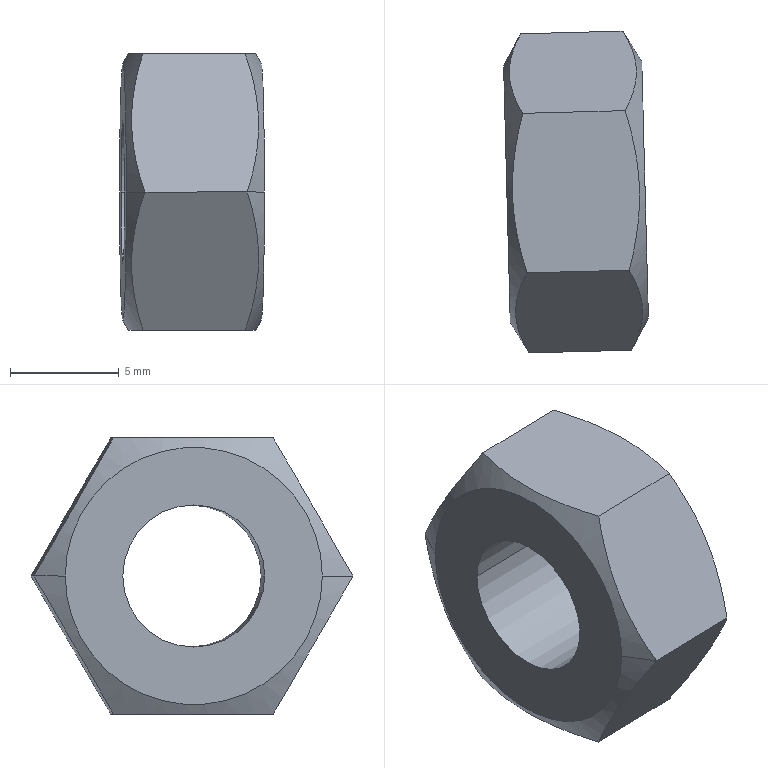Part | STEP file | 1_id1294_x_t | 1 solid | 14 faces | box 6.655 x 14.782 x 12.7 mm | volume 658.806 mm3 | plane 8 | cone 4 | cylinder 2 | commonest cylinder face diameters 6.528 x2